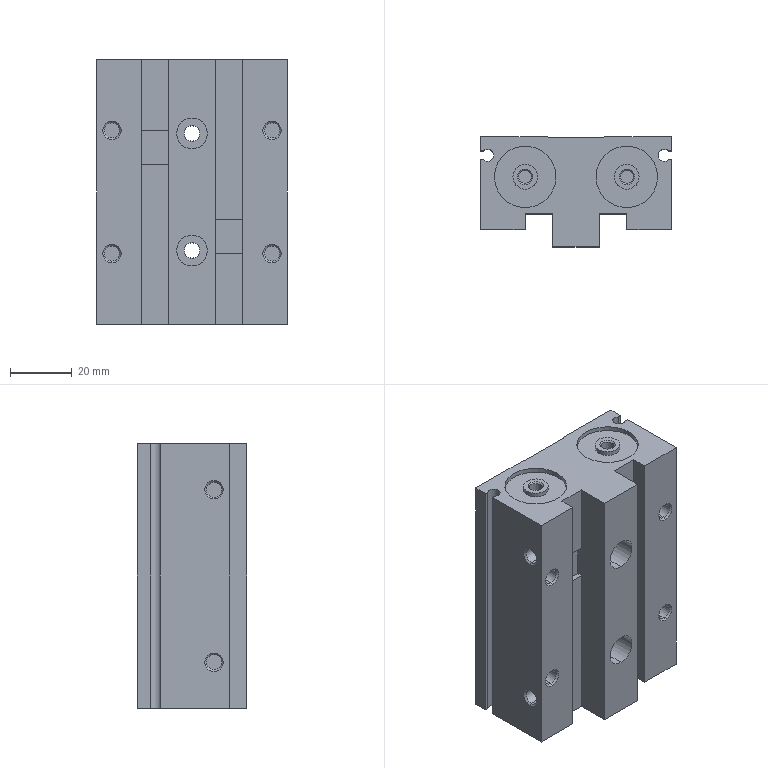Part | SolidWorks | features BaseBody 1 | 1 solid | 132 faces | box 62 x 35.7 x 86 mm | volume 150902 mm3 | plane 56 | cylinder 52 | cone 24 | commonest cylinder face diameters 4.917 x20 20 x8 5 x5 4.134 x4 5.2 x4 8 x4